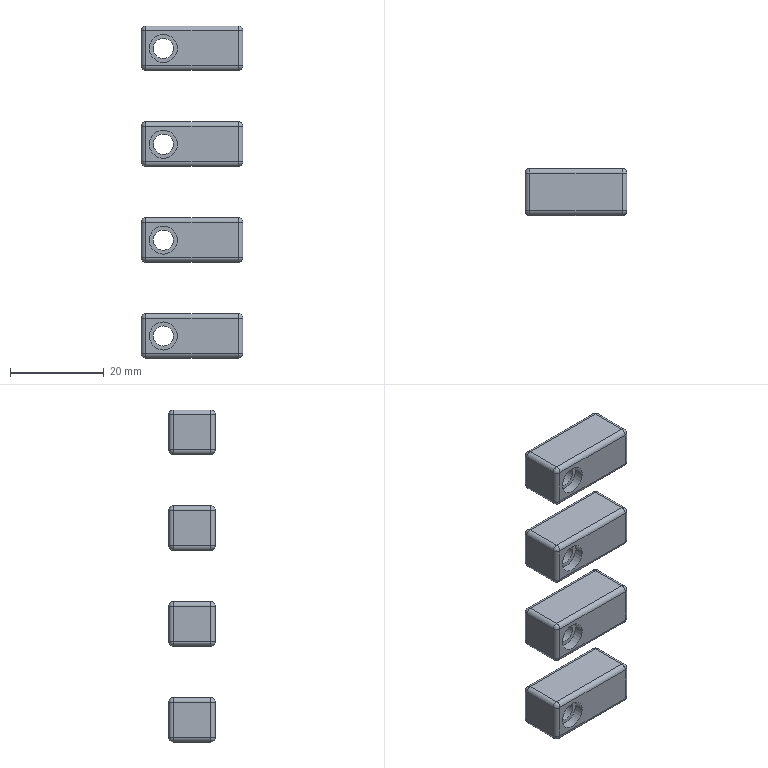CAM job | NX | 3+2 milling, drilling | part box 21.75 x 10 x 71 mm | stock box 26.75 x 12 x 78 mm
Tools:
number,name,description,diameter,corner_radius,flute_length,length,flutes
4,D4,平底铣刀-粗,4.0,0.0,25.0,75.0,2
9,D10,平底铣刀-粗,10.0,0.0,35.0,75.0,2
11,D4-J,平底铣刀-精,4.0,0.0,50.0,75.0,2
10,D10-J,平底铣刀-精,10.0,0.0,35.0,75.0,2
17,D6R0.5,圆鼻刀-粗,6.0,0.5,50.0,75.0,2
1,D80R0.8飞刀,圆鼻刀-粗,80.0,0.8,50.0,75.0,2
1,D80R0.8飞刀-J,圆鼻刀-精,80.0,0.8,50.0,75.0,2
2,D6倒角刀,倒角刀,6.0,0.0,3.0,25.0,2
20,ZT4.3,Drilling Tool,4.3,0.0,50.0,75.0,4
Operations:
program,operation,operation_type,tool,method,geometry_group,spindle_rpm,surface_speed,feed_per_tooth,feed_cut,feed_plunge,cut_length_mm,path_length_mm,cut_time_min,machine_time_min
B,底壁铣飞面一刀开粗_COPY,VolumeBased25DMillingOperation,D80R0.8飞刀,分层开粗-切深K-步距G,W-B,5000.0,1256.637,0.3,3000.0,100.0,716.776,1276.735,0.2389,0.2949
B,底壁铣飞面一刀精光_COPY,VolumeBased25DMillingOperation,D80R0.8飞刀-J,侧刃精光-切深K-步距G,W-B,5000.0,1256.637,0.1,1000.0,100.0,178.998,214.998,0.179,0.1826
B,铣沉头_1,CylinderMilling,D4,METHOD,W-B,6000.0,75.398,0.15,1800.0,100.0,634.307,870.607,0.3524,0.376
B,底壁铣精光侧面-中-选底面_COPY_1,VolumeBased25DMillingOperation,D4-J,侧刃精光-切深K-步距G,W-B,8000.0,100.531,0.0312,500.0,100.0,71.981,248.074,0.144,0.1616
B,等高螺旋爬面_COPY_COPY,ZLevelMilling,D6R0.5,等高爬面-切深K-步距G,W-B,8000.0,150.796,0.3125,5000.0,100.0,7483.947,7734.844,1.497,1.522
B,C0.3封闭铣廓倒角6X45L_COPY,PlanarMilling,D6倒角刀,爬面_倒角-切深0-步距G,W-B,7000.0,131.0,0.1071,1500.0,100.0,128.332,330.543,0.0856,0.1058
A,顶面,FaceMilling,D80R0.8飞刀,侧刃精光-切深K-步距G,W-A,5000.0,1256.637,0.1,1000.0,100.0,165.0,201.0,0.165,0.1686
A,外形粗_2,VolumeBased25DMillingOperation,D10,METHOD,W-A,8000.0,251.327,0.3125,5000.0,80.0,5575.815,5851.031,1.115,1.143
A,沉头孔打点-深0.8,Operation,D6倒角刀,NONE,W-A,8000.0,150.796,0.0312,500.0,90.0,7.2,118.973,0.0144,0.0256
A,沉头孔-钻孔0段,Operation,ZT4.3,NONE,W-A,2800.0,37.825,0.0179,200.0,90.0,56.0,216.573,0.28,0.2961
A,铣孔开粗D4_1,CylinderMilling,D4,NONE,W-A,8000.0,100.531,0.075,1200.0,100.0,222.69,450.19,0.1856,0.2083
A,等高螺旋爬面_COPY,ZLevelMilling,D6R0.5,等高爬面-切深K-步距G,W-A,8000.0,150.796,0.3125,5000.0,100.0,7485.134,7776.345,1.497,1.526
A,铣倒角_1,PlanarMilling,D6倒角刀,NONE,W-A,8000.0,150.796,0.0312,500.0,100.0,110.739,306.185,0.2215,0.241
A,底壁铣精光侧面-中-选底面_COPY,VolumeBased25DMillingOperation,D4-J,侧刃精光-切深K-步距G,W-A,8000.0,100.531,0.0312,500.0,100.0,50.07,202.193,0.1001,0.1154
A,外形半精_2,VolumeBased25DMillingOperation,D10-J,METHOD,W-A,8000.0,251.327,0.0625,1000.0,100.0,391.847,638.556,0.3918,0.4165